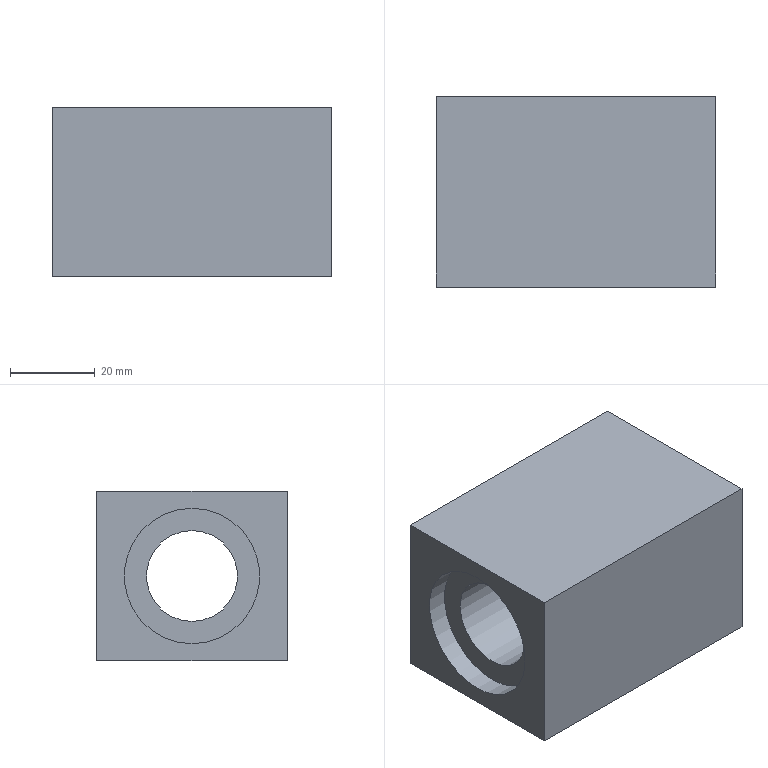Part | STEP file | Tube feed_id826_x_t | 1 solid | 23 faces | box 66 x 45 x 40 mm | volume 90173 mm3 | plane 8 | cone 8 | cylinder 7 | commonest cylinder face diameters 3.3 x4 32 x2 21.5 x1
STEP:
#1=CARTESIAN_POINT('',(0.,0.,0.));
#2=DIRECTION('',(0.,0.,1.));
#3=DIRECTION('',(1.,0.,0.));
#4=AXIS2_PLACEMENT_3D('',#1,#2,#3);
#5=CARTESIAN_POINT('',(-554.,10.056,44.373));
#6=VERTEX_POINT('',#5);
#7=CARTESIAN_POINT('',(-554.,10.056,28.373));
#8=DIRECTION('',(-1.,0.,0.));
#9=DIRECTION('',(0.,0.,1.));
#10=AXIS2_PLACEMENT_3D('',#7,#8,#9);
#11=CIRCLE('',#10,16.);
#12=CARTESIAN_POINT('',(-554.,-12.444,8.1));
#13=DIRECTION('',(1.,0.,0.));
#14=DIRECTION('',(0.,0.,-1.));
#15=AXIS2_PLACEMENT_3D('',#12,#13,#14);
#16=PLANE('',#15);
#17=CARTESIAN_POINT('',(-36.273,22.5));
#18=CARTESIAN_POINT('',(-36.273,50.213));
#19=CARTESIAN_POINT('',(-12.273,36.356));
#20=CARTESIAN_POINT('',(11.727,22.5));
#21=CARTESIAN_POINT('',(-12.273,8.644));
#22=CARTESIAN_POINT('',(-36.273,-5.213));
#23=CARTESIAN_POINT('',(-36.273,22.5));
#24=(BOUNDED_CURVE()B_SPLINE_CURVE(2,(#17,#18,#19,#20,#21,#22,#23),.UNSPECIFIED.,.T.,.F.)B_SPLINE_CURVE_WITH_KNOTS((1,2,2,2,2,1),(-2.094,0.,2.094,4.189,6.283,8.378),.UNSPECIFIED.)CURVE()GEOMETRIC_REPRESENTATION_ITEM()RATIONAL_B_SPLINE_CURVE((1.,0.5,1.,0.5,1.,0.5,1.))REPRESENTATION_ITEM(''));
#25=(GEOMETRIC_REPRESENTATION_CONTEXT(2)PARAMETRIC_REPRESENTATION_CONTEXT()REPRESENTATION_CONTEXT('',''));
#26=DEFINITIONAL_REPRESENTATION('',(#24),#25);
#27=PCURVE('',#16,#26);
#28=CARTESIAN_POINT('',(-554.,10.056,28.373));
#29=DIRECTION('',(-1.,0.,0.));
#30=DIRECTION('',(0.,0.,1.));
#31=AXIS2_PLACEMENT_3D('',#28,#29,#30);
#32=CYLINDRICAL_SURFACE('',#31,16.);
#33=CARTESIAN_POINT('',(0.,0.));
#34=DIRECTION('',(1.,0.));
#35=VECTOR('',#34,1.);
#36=LINE('',#33,#35);
#37=(GEOMETRIC_REPRESENTATION_CONTEXT(2)PARAMETRIC_REPRESENTATION_CONTEXT()REPRESENTATION_CONTEXT('',''));
#38=DEFINITIONAL_REPRESENTATION('',(#36),#37);
#39=PCURVE('',#32,#38);
#40=SURFACE_CURVE('',#11,(#27,#39),.PCURVE_S1.);
#41=EDGE_CURVE('',#6,#6,#40,.T.);
#42=ORIENTED_EDGE('',*,*,#41,.T.);
#43=EDGE_LOOP('',(#42));
#44=FACE_BOUND('',#43,.T.);
#45=CARTESIAN_POINT('',(-554.,-12.444,48.1));
#46=VERTEX_POINT('',#45);
#47=CARTESIAN_POINT('',(-554.,32.556,48.1));
#48=VERTEX_POINT('',#47);
#49=CARTESIAN_POINT('',(-554.,-12.444,48.1));
#50=DIRECTION('',(0.,1.,0.));
#51=VECTOR('',#50,1.);
#52=LINE('',#49,#51);
#53=CARTESIAN_POINT('',(-40.,0.));
#54=DIRECTION('',(0.,1.));
#55=VECTOR('',#54,1.);
#56=LINE('',#53,#55);
#57=(GEOMETRIC_REPRESENTATION_CONTEXT(2)PARAMETRIC_REPRESENTATION_CONTEXT()REPRESENTATION_CONTEXT('',''));
#58=DEFINITIONAL_REPRESENTATION('',(#56),#57);
#59=PCURVE('',#16,#58);
#60=CARTESIAN_POINT('',(-150.,0.,48.1));
#61=DIRECTION('',(0.,0.,1.));
#62=DIRECTION('',(1.,0.,0.));
#63=AXIS2_PLACEMENT_3D('',#60,#61,#62);
#64=PLANE('',#63);
#65=CARTESIAN_POINT('',(-404.,-12.444));
#66=DIRECTION('',(0.,1.));
#67=VECTOR('',#66,1.);
#68=LINE('',#65,#67);
#69=(GEOMETRIC_REPRESENTATION_CONTEXT(2)PARAMETRIC_REPRESENTATION_CONTEXT()REPRESENTATION_CONTEXT('',''));
#70=DEFINITIONAL_REPRESENTATION('',(#68),#69);
#71=PCURVE('',#64,#70);
#72=SURFACE_CURVE('',#52,(#59,#71),.PCURVE_S1.);
#73=EDGE_CURVE('',#46,#48,#72,.T.);
#74=ORIENTED_EDGE('',*,*,#73,.F.);
#75=CARTESIAN_POINT('',(-554.,-12.444,8.1));
#76=VERTEX_POINT('',#75);
#77=CARTESIAN_POINT('',(-554.,-12.444,8.1));
#78=DIRECTION('',(0.,0.,1.));
#79=VECTOR('',#78,1.);
#80=LINE('',#77,#79);
#81=CARTESIAN_POINT('',(0.,0.));
#82=DIRECTION('',(-1.,0.));
#83=VECTOR('',#82,1.);
#84=LINE('',#81,#83);
#85=(GEOMETRIC_REPRESENTATION_CONTEXT(2)PARAMETRIC_REPRESENTATION_CONTEXT()REPRESENTATION_CONTEXT('',''));
#86=DEFINITIONAL_REPRESENTATION('',(#84),#85);
#87=PCURVE('',#16,#86);
#88=CARTESIAN_POINT('',(-620.,-12.444,8.1));
#89=DIRECTION('',(0.,-1.,0.));
#90=DIRECTION('',(0.,0.,-1.));
#91=AXIS2_PLACEMENT_3D('',#88,#89,#90);
#92=PLANE('',#91);
#93=CARTESIAN_POINT('',(0.,66.));
#94=DIRECTION('',(-1.,0.));
#95=VECTOR('',#94,1.);
#96=LINE('',#93,#95);
#97=(GEOMETRIC_REPRESENTATION_CONTEXT(2)PARAMETRIC_REPRESENTATION_CONTEXT()REPRESENTATION_CONTEXT('',''));
#98=DEFINITIONAL_REPRESENTATION('',(#96),#97);
#99=PCURVE('',#92,#98);
#100=SURFACE_CURVE('',#80,(#87,#99),.PCURVE_S1.);
#101=EDGE_CURVE('',#76,#46,#100,.T.);
#102=ORIENTED_EDGE('',*,*,#101,.F.);
#103=CARTESIAN_POINT('',(-554.,32.556,8.1));
#104=VERTEX_POINT('',#103);
#105=CARTESIAN_POINT('',(-554.,-12.444,8.1));
#106=DIRECTION('',(0.,1.,0.));
#107=VECTOR('',#106,1.);
#108=LINE('',#105,#107);
#109=CARTESIAN_POINT('',(0.,0.));
#110=DIRECTION('',(0.,1.));
#111=VECTOR('',#110,1.);
#112=LINE('',#109,#111);
#113=(GEOMETRIC_REPRESENTATION_CONTEXT(2)PARAMETRIC_REPRESENTATION_CONTEXT()REPRESENTATION_CONTEXT('',''));
#114=DEFINITIONAL_REPRESENTATION('',(#112),#113);
#115=PCURVE('',#16,#114);
#116=CARTESIAN_POINT('',(-150.,0.,8.1));
#117=DIRECTION('',(0.,0.,1.));
#118=DIRECTION('',(1.,0.,0.));
#119=AXIS2_PLACEMENT_3D('',#116,#117,#118);
#120=PLANE('',#119);
#121=CARTESIAN_POINT('',(-404.,-12.444));
#122=DIRECTION('',(0.,1.));
#123=VECTOR('',#122,1.);
#124=LINE('',#121,#123);
#125=(GEOMETRIC_REPRESENTATION_CONTEXT(2)PARAMETRIC_REPRESENTATION_CONTEXT()REPRESENTATION_CONTEXT('',''));
#126=DEFINITIONAL_REPRESENTATION('',(#124),#125);
#127=PCURVE('',#120,#126);
#128=SURFACE_CURVE('',#108,(#115,#127),.PCURVE_S1.);
#129=EDGE_CURVE('',#76,#104,#128,.T.);
#130=ORIENTED_EDGE('',*,*,#129,.T.);
#131=CARTESIAN_POINT('',(-554.,32.556,8.1));
#132=DIRECTION('',(0.,0.,1.));
#133=VECTOR('',#132,1.);
#134=LINE('',#131,#133);
#135=CARTESIAN_POINT('',(0.,45.));
#136=DIRECTION('',(-1.,0.));
#137=VECTOR('',#136,1.);
#138=LINE('',#135,#137);
#139=(GEOMETRIC_REPRESENTATION_CONTEXT(2)PARAMETRIC_REPRESENTATION_CONTEXT()REPRESENTATION_CONTEXT('',''));
#140=DEFINITIONAL_REPRESENTATION('',(#138),#139);
#141=PCURVE('',#16,#140);
#142=CARTESIAN_POINT('',(-554.,32.556,8.1));
#143=DIRECTION('',(0.,1.,0.));
#144=DIRECTION('',(0.,0.,1.));
#145=AXIS2_PLACEMENT_3D('',#142,#143,#144);
#146=PLANE('',#145);
#147=CARTESIAN_POINT('',(0.,0.));
#148=DIRECTION('',(1.,0.));
#149=VECTOR('',#148,1.);
#150=LINE('',#147,#149);
#151=(GEOMETRIC_REPRESENTATION_CONTEXT(2)PARAMETRIC_REPRESENTATION_CONTEXT()REPRESENTATION_CONTEXT('',''));
#152=DEFINITIONAL_REPRESENTATION('',(#150),#151);
#153=PCURVE('',#146,#152);
#154=SURFACE_CURVE('',#134,(#141,#153),.PCURVE_S1.);
#155=EDGE_CURVE('',#104,#48,#154,.T.);
#156=ORIENTED_EDGE('',*,*,#155,.T.);
#157=EDGE_LOOP('',(#74,#102,#130,#156));
#158=FACE_BOUND('',#157,.T.);
#159=ADVANCED_FACE('',(#44,#158),#16,.T.);
#160=CARTESIAN_POINT('',(-620.,32.556,48.1));
#161=VERTEX_POINT('',#160);
#162=CARTESIAN_POINT('',(-554.,32.556,48.1));
#163=DIRECTION('',(-1.,0.,0.));
#164=VECTOR('',#163,1.);
#165=LINE('',#162,#164);
#166=CARTESIAN_POINT('',(40.,0.));
#167=DIRECTION('',(0.,-1.));
#168=VECTOR('',#167,1.);
#169=LINE('',#166,#168);
#170=(GEOMETRIC_REPRESENTATION_CONTEXT(2)PARAMETRIC_REPRESENTATION_CONTEXT()REPRESENTATION_CONTEXT('',''));
#171=DEFINITIONAL_REPRESENTATION('',(#169),#170);
#172=PCURVE('',#146,#171);
#173=CARTESIAN_POINT('',(-404.,32.556));
#174=DIRECTION('',(-1.,0.));
#175=VECTOR('',#174,1.);
#176=LINE('',#173,#175);
#177=(GEOMETRIC_REPRESENTATION_CONTEXT(2)PARAMETRIC_REPRESENTATION_CONTEXT()REPRESENTATION_CONTEXT('',''));
#178=DEFINITIONAL_REPRESENTATION('',(#176),#177);
#179=PCURVE('',#64,#178);
#180=SURFACE_CURVE('',#165,(#172,#179),.PCURVE_S1.);
#181=EDGE_CURVE('',#48,#161,#180,.T.);
#182=ORIENTED_EDGE('',*,*,#181,.F.);
#183=ORIENTED_EDGE('',*,*,#155,.F.);
#184=CARTESIAN_POINT('',(-620.,32.556,8.1));
#185=VERTEX_POINT('',#184);
#186=CARTESIAN_POINT('',(-554.,32.556,8.1));
#187=DIRECTION('',(-1.,0.,0.));
#188=VECTOR('',#187,1.);
#189=LINE('',#186,#188);
#190=CARTESIAN_POINT('',(0.,0.));
#191=DIRECTION('',(0.,-1.));
#192=VECTOR('',#191,1.);
#193=LINE('',#190,#192);
#194=(GEOMETRIC_REPRESENTATION_CONTEXT(2)PARAMETRIC_REPRESENTATION_CONTEXT()REPRESENTATION_CONTEXT('',''));
#195=DEFINITIONAL_REPRESENTATION('',(#193),#194);
#196=PCURVE('',#146,#195);
#197=CARTESIAN_POINT('',(-404.,32.556));
#198=DIRECTION('',(-1.,0.));
#199=VECTOR('',#198,1.);
#200=LINE('',#197,#199);
#201=(GEOMETRIC_REPRESENTATION_CONTEXT(2)PARAMETRIC_REPRESENTATION_CONTEXT()REPRESENTATION_CONTEXT('',''));
#202=DEFINITIONAL_REPRESENTATION('',(#200),#201);
#203=PCURVE('',#120,#202);
#204=SURFACE_CURVE('',#189,(#196,#203),.PCURVE_S1.);
#205=EDGE_CURVE('',#104,#185,#204,.T.);
#206=ORIENTED_EDGE('',*,*,#205,.T.);
#207=CARTESIAN_POINT('',(-620.,32.556,8.1));
#208=DIRECTION('',(0.,0.,1.));
#209=VECTOR('',#208,1.);
#210=LINE('',#207,#209);
#211=CARTESIAN_POINT('',(0.,-66.));
#212=DIRECTION('',(1.,0.));
#213=VECTOR('',#212,1.);
#214=LINE('',#211,#213);
#215=(GEOMETRIC_REPRESENTATION_CONTEXT(2)PARAMETRIC_REPRESENTATION_CONTEXT()REPRESENTATION_CONTEXT('',''));
#216=DEFINITIONAL_REPRESENTATION('',(#214),#215);
#217=PCURVE('',#146,#216);
#218=CARTESIAN_POINT('',(-620.,32.556,8.1));
#219=DIRECTION('',(-1.,0.,0.));
#220=DIRECTION('',(0.,0.,1.));
#221=AXIS2_PLACEMENT_3D('',#218,#219,#220);
#222=PLANE('',#221);
#223=CARTESIAN_POINT('',(0.,0.));
#224=DIRECTION('',(1.,0.));
#225=VECTOR('',#224,1.);
#226=LINE('',#223,#225);
#227=(GEOMETRIC_REPRESENTATION_CONTEXT(2)PARAMETRIC_REPRESENTATION_CONTEXT()REPRESENTATION_CONTEXT('',''));
#228=DEFINITIONAL_REPRESENTATION('',(#226),#227);
#229=PCURVE('',#222,#228);
#230=SURFACE_CURVE('',#210,(#217,#229),.PCURVE_S1.);
#231=EDGE_CURVE('',#185,#161,#230,.T.);
#232=ORIENTED_EDGE('',*,*,#231,.T.);
#233=EDGE_LOOP('',(#182,#183,#206,#232));
#234=FACE_BOUND('',#233,.T.);
#235=ADVANCED_FACE('',(#234),#146,.T.);
#236=CARTESIAN_POINT('',(-620.,10.056,12.1));
#237=VERTEX_POINT('',#236);
#238=CARTESIAN_POINT('',(-620.,10.056,28.1));
#239=DIRECTION('',(1.,0.,0.));
#240=DIRECTION('',(0.,0.,-1.));
#241=AXIS2_PLACEMENT_3D('',#238,#239,#240);
#242=CIRCLE('',#241,16.);
#243=CARTESIAN_POINT('',(4.,-22.5));
#244=CARTESIAN_POINT('',(4.,5.213));
#245=CARTESIAN_POINT('',(28.,-8.644));
#246=CARTESIAN_POINT('',(52.,-22.5));
#247=CARTESIAN_POINT('',(28.,-36.356));
#248=CARTESIAN_POINT('',(4.,-50.213));
#249=CARTESIAN_POINT('',(4.,-22.5));
#250=(BOUNDED_CURVE()B_SPLINE_CURVE(2,(#243,#244,#245,#246,#247,#248,#249),.UNSPECIFIED.,.T.,.F.)B_SPLINE_CURVE_WITH_KNOTS((1,2,2,2,2,1),(-2.094,0.,2.094,4.189,6.283,8.378),.UNSPECIFIED.)CURVE()GEOMETRIC_REPRESENTATION_ITEM()RATIONAL_B_SPLINE_CURVE((1.,0.5,1.,0.5,1.,0.5,1.))REPRESENTATION_ITEM(''));
#251=(GEOMETRIC_REPRESENTATION_CONTEXT(2)PARAMETRIC_REPRESENTATION_CONTEXT()REPRESENTATION_CONTEXT('',''));
#252=DEFINITIONAL_REPRESENTATION('',(#250),#251);
#253=PCURVE('',#222,#252);
#254=CARTESIAN_POINT('',(-620.,10.056,28.1));
#255=DIRECTION('',(1.,0.,0.));
#256=DIRECTION('',(0.,0.,-1.));
#257=AXIS2_PLACEMENT_3D('',#254,#255,#256);
#258=CYLINDRICAL_SURFACE('',#257,16.);
#259=CARTESIAN_POINT('',(0.,0.));
#260=DIRECTION('',(1.,0.));
#261=VECTOR('',#260,1.);
#262=LINE('',#259,#261);
#263=(GEOMETRIC_REPRESENTATION_CONTEXT(2)PARAMETRIC_REPRESENTATION_CONTEXT()REPRESENTATION_CONTEXT('',''));
#264=DEFINITIONAL_REPRESENTATION('',(#262),#263);
#265=PCURVE('',#258,#264);
#266=SURFACE_CURVE('',#242,(#253,#265),.PCURVE_S1.);
#267=EDGE_CURVE('',#237,#237,#266,.T.);
#268=ORIENTED_EDGE('',*,*,#267,.T.);
#269=EDGE_LOOP('',(#268));
#270=FACE_BOUND('',#269,.T.);
#271=CARTESIAN_POINT('',(-620.,-12.444,48.1));
#272=VERTEX_POINT('',#271);
#273=CARTESIAN_POINT('',(-620.,32.556,48.1));
#274=DIRECTION('',(0.,-1.,0.));
#275=VECTOR('',#274,1.);
#276=LINE('',#273,#275);
#277=CARTESIAN_POINT('',(40.,0.));
#278=DIRECTION('',(0.,-1.));
#279=VECTOR('',#278,1.);
#280=LINE('',#277,#279);
#281=(GEOMETRIC_REPRESENTATION_CONTEXT(2)PARAMETRIC_REPRESENTATION_CONTEXT()REPRESENTATION_CONTEXT('',''));
#282=DEFINITIONAL_REPRESENTATION('',(#280),#281);
#283=PCURVE('',#222,#282);
#284=CARTESIAN_POINT('',(-470.,32.556));
#285=DIRECTION('',(0.,-1.));
#286=VECTOR('',#285,1.);
#287=LINE('',#284,#286);
#288=(GEOMETRIC_REPRESENTATION_CONTEXT(2)PARAMETRIC_REPRESENTATION_CONTEXT()REPRESENTATION_CONTEXT('',''));
#289=DEFINITIONAL_REPRESENTATION('',(#287),#288);
#290=PCURVE('',#64,#289);
#291=SURFACE_CURVE('',#276,(#283,#290),.PCURVE_S1.);
#292=EDGE_CURVE('',#161,#272,#291,.T.);
#293=ORIENTED_EDGE('',*,*,#292,.F.);
#294=ORIENTED_EDGE('',*,*,#231,.F.);
#295=CARTESIAN_POINT('',(-620.,-12.444,8.1));
#296=VERTEX_POINT('',#295);
#297=CARTESIAN_POINT('',(-620.,32.556,8.1));
#298=DIRECTION('',(0.,-1.,0.));
#299=VECTOR('',#298,1.);
#300=LINE('',#297,#299);
#301=CARTESIAN_POINT('',(0.,0.));
#302=DIRECTION('',(0.,-1.));
#303=VECTOR('',#302,1.);
#304=LINE('',#301,#303);
#305=(GEOMETRIC_REPRESENTATION_CONTEXT(2)PARAMETRIC_REPRESENTATION_CONTEXT()REPRESENTATION_CONTEXT('',''));
#306=DEFINITIONAL_REPRESENTATION('',(#304),#305);
#307=PCURVE('',#222,#306);
#308=CARTESIAN_POINT('',(-470.,32.556));
#309=DIRECTION('',(0.,-1.));
#310=VECTOR('',#309,1.);
#311=LINE('',#308,#310);
#312=(GEOMETRIC_REPRESENTATION_CONTEXT(2)PARAMETRIC_REPRESENTATION_CONTEXT()REPRESENTATION_CONTEXT('',''));
#313=DEFINITIONAL_REPRESENTATION('',(#311),#312);
#314=PCURVE('',#120,#313);
#315=SURFACE_CURVE('',#300,(#307,#314),.PCURVE_S1.);
#316=EDGE_CURVE('',#185,#296,#315,.T.);
#317=ORIENTED_EDGE('',*,*,#316,.T.);
#318=CARTESIAN_POINT('',(-620.,-12.444,8.1));
#319=DIRECTION('',(0.,0.,1.));
#320=VECTOR('',#319,1.);
#321=LINE('',#318,#320);
#322=CARTESIAN_POINT('',(0.,-45.));
#323=DIRECTION('',(1.,0.));
#324=VECTOR('',#323,1.);
#325=LINE('',#322,#324);
#326=(GEOMETRIC_REPRESENTATION_CONTEXT(2)PARAMETRIC_REPRESENTATION_CONTEXT()REPRESENTATION_CONTEXT('',''));
#327=DEFINITIONAL_REPRESENTATION('',(#325),#326);
#328=PCURVE('',#222,#327);
#329=CARTESIAN_POINT('',(0.,0.));
#330=DIRECTION('',(-1.,0.));
#331=VECTOR('',#330,1.);
#332=LINE('',#329,#331);
#333=(GEOMETRIC_REPRESENTATION_CONTEXT(2)PARAMETRIC_REPRESENTATION_CONTEXT()REPRESENTATION_CONTEXT('',''));
#334=DEFINITIONAL_REPRESENTATION('',(#332),#333);
#335=PCURVE('',#92,#334);
#336=SURFACE_CURVE('',#321,(#328,#335),.PCURVE_S1.);
#337=EDGE_CURVE('',#296,#272,#336,.T.);
#338=ORIENTED_EDGE('',*,*,#337,.T.);
#339=EDGE_LOOP('',(#293,#294,#317,#338));
#340=FACE_BOUND('',#339,.T.);
#341=ADVANCED_FACE('',(#270,#340),#222,.T.);
#342=CARTESIAN_POINT('',(-620.,-12.444,48.1));
#343=DIRECTION('',(1.,0.,0.));
#344=VECTOR('',#343,1.);
#345=LINE('',#342,#344);
#346=CARTESIAN_POINT('',(-40.,0.));
#347=DIRECTION('',(0.,1.));
#348=VECTOR('',#347,1.);
#349=LINE('',#346,#348);
#350=(GEOMETRIC_REPRESENTATION_CONTEXT(2)PARAMETRIC_REPRESENTATION_CONTEXT()REPRESENTATION_CONTEXT('',''));
#351=DEFINITIONAL_REPRESENTATION('',(#349),#350);
#352=PCURVE('',#92,#351);
#353=CARTESIAN_POINT('',(-470.,-12.444));
#354=DIRECTION('',(1.,0.));
#355=VECTOR('',#354,1.);
#356=LINE('',#353,#355);
#357=(GEOMETRIC_REPRESENTATION_CONTEXT(2)PARAMETRIC_REPRESENTATION_CONTEXT()REPRESENTATION_CONTEXT('',''));
#358=DEFINITIONAL_REPRESENTATION('',(#356),#357);
#359=PCURVE('',#64,#358);
#360=SURFACE_CURVE('',#345,(#352,#359),.PCURVE_S1.);
#361=EDGE_CURVE('',#272,#46,#360,.T.);
#362=ORIENTED_EDGE('',*,*,#361,.F.);
#363=ORIENTED_EDGE('',*,*,#337,.F.);
#364=CARTESIAN_POINT('',(-620.,-12.444,8.1));
#365=DIRECTION('',(1.,0.,0.));
#366=VECTOR('',#365,1.);
#367=LINE('',#364,#366);
#368=CARTESIAN_POINT('',(0.,0.));
#369=DIRECTION('',(0.,1.));
#370=VECTOR('',#369,1.);
#371=LINE('',#368,#370);
#372=(GEOMETRIC_REPRESENTATION_CONTEXT(2)PARAMETRIC_REPRESENTATION_CONTEXT()REPRESENTATION_CONTEXT('',''));
#373=DEFINITIONAL_REPRESENTATION('',(#371),#372);
#374=PCURVE('',#92,#373);
#375=CARTESIAN_POINT('',(-470.,-12.444));
#376=DIRECTION('',(1.,0.));
#377=VECTOR('',#376,1.);
#378=LINE('',#375,#377);
#379=(GEOMETRIC_REPRESENTATION_CONTEXT(2)PARAMETRIC_REPRESENTATION_CONTEXT()REPRESENTATION_CONTEXT('',''));
#380=DEFINITIONAL_REPRESENTATION('',(#378),#379);
#381=PCURVE('',#120,#380);
#382=SURFACE_CURVE('',#367,(#374,#381),.PCURVE_S1.);
#383=EDGE_CURVE('',#296,#76,#382,.T.);
#384=ORIENTED_EDGE('',*,*,#383,.T.);
#385=ORIENTED_EDGE('',*,*,#101,.T.);
#386=EDGE_LOOP('',(#362,#363,#384,#385));
#387=FACE_BOUND('',#386,.T.);
#388=ADVANCED_FACE('',(#387),#92,.T.);
#389=CARTESIAN_POINT('',(-610.,22.556,8.1));
#390=VERTEX_POINT('',#389);
#391=CARTESIAN_POINT('',(-612.,22.556,8.1));
#392=DIRECTION('',(0.,0.,1.));
#393=DIRECTION('',(1.,0.,0.));
#394=AXIS2_PLACEMENT_3D('',#391,#392,#393);
#395=CIRCLE('',#394,2.);
#396=CARTESIAN_POINT('',(-462.,22.556));
#397=DIRECTION('',(1.,0.));
#398=AXIS2_PLACEMENT_2D('',#396,#397);
#399=CIRCLE('',#398,2.);
#400=(GEOMETRIC_REPRESENTATION_CONTEXT(2)PARAMETRIC_REPRESENTATION_CONTEXT()REPRESENTATION_CONTEXT('',''));
#401=DEFINITIONAL_REPRESENTATION('',(#399),#400);
#402=PCURVE('',#120,#401);
#403=CARTESIAN_POINT('',(-612.,22.556,8.1));
#404=DIRECTION('',(0.,0.,-1.));
#405=DIRECTION('',(-1.,0.,0.));
#406=AXIS2_PLACEMENT_3D('',#403,#404,#405);
#407=CONICAL_SURFACE('',#406,2.,0.7854);
#408=CARTESIAN_POINT('',(9.425,0.));
#409=DIRECTION('',(-1.,0.));
#410=VECTOR('',#409,1.);
#411=LINE('',#408,#410);
#412=(GEOMETRIC_REPRESENTATION_CONTEXT(2)PARAMETRIC_REPRESENTATION_CONTEXT()REPRESENTATION_CONTEXT('',''));
#413=DEFINITIONAL_REPRESENTATION('',(#411),#412);
#414=PCURVE('',#407,#413);
#415=SURFACE_CURVE('',#395,(#402,#414),.PCURVE_S1.);
#416=EDGE_CURVE('',#390,#390,#415,.T.);
#417=ORIENTED_EDGE('',*,*,#416,.T.);
#418=EDGE_LOOP('',(#417));
#419=FACE_BOUND('',#418,.T.);
#420=CARTESIAN_POINT('',(-560.,22.556,8.1));
#421=VERTEX_POINT('',#420);
#422=CARTESIAN_POINT('',(-562.,22.556,8.1));
#423=DIRECTION('',(0.,0.,1.));
#424=DIRECTION('',(1.,0.,0.));
#425=AXIS2_PLACEMENT_3D('',#422,#423,#424);
#426=CIRCLE('',#425,2.);
#427=CARTESIAN_POINT('',(-412.,22.556));
#428=DIRECTION('',(1.,0.));
#429=AXIS2_PLACEMENT_2D('',#427,#428);
#430=CIRCLE('',#429,2.);
#431=(GEOMETRIC_REPRESENTATION_CONTEXT(2)PARAMETRIC_REPRESENTATION_CONTEXT()REPRESENTATION_CONTEXT('',''));
#432=DEFINITIONAL_REPRESENTATION('',(#430),#431);
#433=PCURVE('',#120,#432);
#434=CARTESIAN_POINT('',(-562.,22.556,8.1));
#435=DIRECTION('',(0.,0.,-1.));
#436=DIRECTION('',(-1.,0.,0.));
#437=AXIS2_PLACEMENT_3D('',#434,#435,#436);
#438=CONICAL_SURFACE('',#437,2.,0.7854);
#439=CARTESIAN_POINT('',(9.425,0.));
#440=DIRECTION('',(-1.,0.));
#441=VECTOR('',#440,1.);
#442=LINE('',#439,#441);
#443=(GEOMETRIC_REPRESENTATION_CONTEXT(2)PARAMETRIC_REPRESENTATION_CONTEXT()REPRESENTATION_CONTEXT('',''));
#444=DEFINITIONAL_REPRESENTATION('',(#442),#443);
#445=PCURVE('',#438,#444);
#446=SURFACE_CURVE('',#426,(#433,#445),.PCURVE_S1.);
#447=EDGE_CURVE('',#421,#421,#446,.T.);
#448=ORIENTED_EDGE('',*,*,#447,.T.);
#449=EDGE_LOOP('',(#448));
#450=FACE_BOUND('',#449,.T.);
#451=CARTESIAN_POINT('',(-560.,-2.444,8.1));
#452=VERTEX_POINT('',#451);
#453=CARTESIAN_POINT('',(-562.,-2.444,8.1));
#454=DIRECTION('',(0.,0.,1.));
#455=DIRECTION('',(1.,0.,0.));
#456=AXIS2_PLACEMENT_3D('',#453,#454,#455);
#457=CIRCLE('',#456,2.);
#458=CARTESIAN_POINT('',(-412.,-2.444));
#459=DIRECTION('',(1.,0.));
#460=AXIS2_PLACEMENT_2D('',#458,#459);
#461=CIRCLE('',#460,2.);
#462=(GEOMETRIC_REPRESENTATION_CONTEXT(2)PARAMETRIC_REPRESENTATION_CONTEXT()REPRESENTATION_CONTEXT('',''));
#463=DEFINITIONAL_REPRESENTATION('',(#461),#462);
#464=PCURVE('',#120,#463);
#465=CARTESIAN_POINT('',(-562.,-2.444,8.1));
#466=DIRECTION('',(0.,0.,-1.));
#467=DIRECTION('',(-1.,0.,0.));
#468=AXIS2_PLACEMENT_3D('',#465,#466,#467);
#469=CONICAL_SURFACE('',#468,2.,0.7854);
#470=CARTESIAN_POINT('',(9.425,0.));
#471=DIRECTION('',(-1.,0.));
#472=VECTOR('',#471,1.);
#473=LINE('',#470,#472);
#474=(GEOMETRIC_REPRESENTATION_CONTEXT(2)PARAMETRIC_REPRESENTATION_CONTEXT()REPRESENTATION_CONTEXT('',''));
#475=DEFINITIONAL_REPRESENTATION('',(#473),#474);
#476=PCURVE('',#469,#475);
#477=SURFACE_CURVE('',#457,(#464,#476),.PCURVE_S1.);
#478=EDGE_CURVE('',#452,#452,#477,.T.);
#479=ORIENTED_EDGE('',*,*,#478,.T.);
#480=EDGE_LOOP('',(#479));
#481=FACE_BOUND('',#480,.T.);
#482=CARTESIAN_POINT('',(-610.,-2.444,8.1));
#483=VERTEX_POINT('',#482);
#484=CARTESIAN_POINT('',(-612.,-2.444,8.1));
#485=DIRECTION('',(0.,0.,1.));
#486=DIRECTION('',(1.,0.,0.));
#487=AXIS2_PLACEMENT_3D('',#484,#485,#486);
#488=CIRCLE('',#487,2.);
#489=CARTESIAN_POINT('',(-462.,-2.444));
#490=DIRECTION('',(1.,0.));
#491=AXIS2_PLACEMENT_2D('',#489,#490);
#492=CIRCLE('',#491,2.);
#493=(GEOMETRIC_REPRESENTATION_CONTEXT(2)PARAMETRIC_REPRESENTATION_CONTEXT()REPRESENTATION_CONTEXT('',''));
#494=DEFINITIONAL_REPRESENTATION('',(#492),#493);
#495=PCURVE('',#120,#494);
#496=CARTESIAN_POINT('',(-612.,-2.444,8.1));
#497=DIRECTION('',(0.,0.,-1.));
#498=DIRECTION('',(-1.,0.,0.));
#499=AXIS2_PLACEMENT_3D('',#496,#497,#498);
#500=CONICAL_SURFACE('',#499,2.,0.7854);
#501=CARTESIAN_POINT('',(9.425,0.));
#502=DIRECTION('',(-1.,0.));
#503=VECTOR('',#502,1.);
#504=LINE('',#501,#503);
#505=(GEOMETRIC_REPRESENTATION_CONTEXT(2)PARAMETRIC_REPRESENTATION_CONTEXT()REPRESENTATION_CONTEXT('',''));
#506=DEFINITIONAL_REPRESENTATION('',(#504),#505);
#507=PCURVE('',#500,#506);
#508=SURFACE_CURVE('',#488,(#495,#507),.PCURVE_S1.);
#509=EDGE_CURVE('',#483,#483,#508,.T.);
#510=ORIENTED_EDGE('',*,*,#509,.T.);
#511=EDGE_LOOP('',(#510));
#512=FACE_BOUND('',#511,.T.);
#513=ORIENTED_EDGE('',*,*,#129,.F.);
#514=ORIENTED_EDGE('',*,*,#383,.F.);
#515=ORIENTED_EDGE('',*,*,#316,.F.);
#516=ORIENTED_EDGE('',*,*,#205,.F.);
#517=EDGE_LOOP('',(#513,#514,#515,#516));
#518=FACE_BOUND('',#517,.T.);
#519=ADVANCED_FACE('',(#419,#450,#481,#512,#518),#120,.F.);
#520=ORIENTED_EDGE('',*,*,#73,.T.);
#521=ORIENTED_EDGE('',*,*,#181,.T.);
#522=ORIENTED_EDGE('',*,*,#292,.T.);
#523=ORIENTED_EDGE('',*,*,#361,.T.);
#524=EDGE_LOOP('',(#520,#521,#522,#523));
#525=FACE_BOUND('',#524,.T.);
#526=ADVANCED_FACE('',(#525),#64,.T.);
#527=CARTESIAN_POINT('',(-559.,10.056,38.85));
#528=VERTEX_POINT('',#527);
#529=CARTESIAN_POINT('',(-559.,10.056,17.35));
#530=VERTEX_POINT('',#529);
#531=CARTESIAN_POINT('',(-559.,10.056,28.1));
#532=DIRECTION('',(-1.,0.,0.));
#533=DIRECTION('',(0.,0.,1.));
#534=AXIS2_PLACEMENT_3D('',#531,#532,#533);
#535=CIRCLE('',#534,10.75);
#536=CARTESIAN_POINT('',(-559.,10.056,28.373));
#537=DIRECTION('',(-1.,0.,0.));
#538=DIRECTION('',(0.,0.,1.));
#539=AXIS2_PLACEMENT_3D('',#536,#537,#538);
#540=PLANE('',#539);
#541=CARTESIAN_POINT('',(-0.2729,0.));
#542=DIRECTION('',(1.,0.));
#543=AXIS2_PLACEMENT_2D('',#541,#542);
#544=CIRCLE('',#543,10.75);
#545=(GEOMETRIC_REPRESENTATION_CONTEXT(2)PARAMETRIC_REPRESENTATION_CONTEXT()REPRESENTATION_CONTEXT('',''));
#546=DEFINITIONAL_REPRESENTATION('',(#544),#545);
#547=PCURVE('',#540,#546);
#548=CARTESIAN_POINT('',(-615.,10.056,28.1));
#549=DIRECTION('',(1.,0.,0.));
#550=DIRECTION('',(0.,0.,-1.));
#551=AXIS2_PLACEMENT_3D('',#548,#549,#550);
#552=CYLINDRICAL_SURFACE('',#551,10.75);
#553=CARTESIAN_POINT('',(3.142,56.));
#554=DIRECTION('',(-1.,0.));
#555=VECTOR('',#554,1.);
#556=LINE('',#553,#555);
#557=(GEOMETRIC_REPRESENTATION_CONTEXT(2)PARAMETRIC_REPRESENTATION_CONTEXT()REPRESENTATION_CONTEXT('',''));
#558=DEFINITIONAL_REPRESENTATION('',(#556),#557);
#559=PCURVE('',#552,#558);
#560=SURFACE_CURVE('',#535,(#547,#559),.PCURVE_S1.);
#561=EDGE_CURVE('',#528,#530,#560,.T.);
#562=ORIENTED_EDGE('',*,*,#561,.T.);
#563=CARTESIAN_POINT('',(-559.,10.056,28.1));
#564=DIRECTION('',(-1.,0.,0.));
#565=DIRECTION('',(0.,0.,1.));
#566=AXIS2_PLACEMENT_3D('',#563,#564,#565);
#567=CIRCLE('',#566,10.75);
#568=CARTESIAN_POINT('',(-0.2729,0.));
#569=DIRECTION('',(1.,0.));
#570=AXIS2_PLACEMENT_2D('',#568,#569);
#571=CIRCLE('',#570,10.75);
#572=(GEOMETRIC_REPRESENTATION_CONTEXT(2)PARAMETRIC_REPRESENTATION_CONTEXT()REPRESENTATION_CONTEXT('',''));
#573=DEFINITIONAL_REPRESENTATION('',(#571),#572);
#574=PCURVE('',#540,#573);
#575=CARTESIAN_POINT('',(9.425,56.));
#576=DIRECTION('',(-1.,0.));
#577=VECTOR('',#576,1.);
#578=LINE('',#575,#577);
#579=(GEOMETRIC_REPRESENTATION_CONTEXT(2)PARAMETRIC_REPRESENTATION_CONTEXT()REPRESENTATION_CONTEXT('',''));
#580=DEFINITIONAL_REPRESENTATION('',(#578),#579);
#581=PCURVE('',#552,#580);
#582=SURFACE_CURVE('',#567,(#574,#581),.PCURVE_S1.);
#583=EDGE_CURVE('',#530,#528,#582,.T.);
#584=ORIENTED_EDGE('',*,*,#583,.T.);
#585=EDGE_LOOP('',(#562,#584));
#586=FACE_BOUND('',#585,.T.);
#587=CARTESIAN_POINT('',(-559.,10.056,44.373));
#588=VERTEX_POINT('',#587);
#589=CARTESIAN_POINT('',(-559.,10.056,28.373));
#590=DIRECTION('',(-1.,0.,0.));
#591=DIRECTION('',(0.,0.,1.));
#592=AXIS2_PLACEMENT_3D('',#589,#590,#591);
#593=CIRCLE('',#592,16.);
#594=CARTESIAN_POINT('',(0.,0.));
#595=DIRECTION('',(1.,0.));
#596=AXIS2_PLACEMENT_2D('',#594,#595);
#597=CIRCLE('',#596,16.);
#598=(GEOMETRIC_REPRESENTATION_CONTEXT(2)PARAMETRIC_REPRESENTATION_CONTEXT()REPRESENTATION_CONTEXT('',''));
#599=DEFINITIONAL_REPRESENTATION('',(#597),#598);
#600=PCURVE('',#540,#599);
#601=CARTESIAN_POINT('',(0.,5.));
#602=DIRECTION('',(1.,0.));
#603=VECTOR('',#602,1.);
#604=LINE('',#601,#603);
#605=(GEOMETRIC_REPRESENTATION_CONTEXT(2)PARAMETRIC_REPRESENTATION_CONTEXT()REPRESENTATION_CONTEXT('',''));
#606=DEFINITIONAL_REPRESENTATION('',(#604),#605);
#607=PCURVE('',#32,#606);
#608=SURFACE_CURVE('',#593,(#600,#607),.PCURVE_S1.);
#609=EDGE_CURVE('',#588,#588,#608,.T.);
#610=ORIENTED_EDGE('',*,*,#609,.F.);
#611=EDGE_LOOP('',(#610));
#612=FACE_BOUND('',#611,.T.);
#613=ADVANCED_FACE('',(#586,#612),#540,.F.);
#614=ORIENTED_EDGE('',*,*,#609,.F.);
#615=CARTESIAN_POINT('',(-554.,10.056,44.373));
#616=CARTESIAN_POINT('',(-559.,10.056,44.373));
#617=B_SPLINE_CURVE_WITH_KNOTS('',1,(#615,#616),.UNSPECIFIED.,.F.,.F.,(2,2),(0.,5.),.PIECEWISE_BEZIER_KNOTS.);
#618=CARTESIAN_POINT('',(0.,0.));
#619=DIRECTION('',(0.,1.));
#620=VECTOR('',#619,1.);
#621=LINE('',#618,#620);
#622=(GEOMETRIC_REPRESENTATION_CONTEXT(2)PARAMETRIC_REPRESENTATION_CONTEXT()REPRESENTATION_CONTEXT('',''));
#623=DEFINITIONAL_REPRESENTATION('',(#621),#622);
#624=PCURVE('',#32,#623);
#625=CARTESIAN_POINT('',(6.283,0.));
#626=DIRECTION('',(0.,1.));
#627=VECTOR('',#626,1.);
#628=LINE('',#625,#627);
#629=(GEOMETRIC_REPRESENTATION_CONTEXT(2)PARAMETRIC_REPRESENTATION_CONTEXT()REPRESENTATION_CONTEXT('',''));
#630=DEFINITIONAL_REPRESENTATION('',(#628),#629);
#631=PCURVE('',#32,#630);
#632=SEAM_CURVE('',#617,(#624,#631),.PCURVE_S1.);
#633=EDGE_CURVE('',#6,#588,#632,.T.);
#634=ORIENTED_EDGE('',*,*,#633,.F.);
#635=ORIENTED_EDGE('',*,*,#41,.T.);
#636=ORIENTED_EDGE('',*,*,#633,.T.);
#637=EDGE_LOOP('',(#614,#634,#635,#636));
#638=FACE_BOUND('',#637,.F.);
#639=ADVANCED_FACE('',(#638),#32,.F.);
#640=CARTESIAN_POINT('',(-615.,10.056,17.35));
#641=VERTEX_POINT('',#640);
#642=CARTESIAN_POINT('',(-615.,10.056,28.1));
#643=DIRECTION('',(1.,0.,0.));
#644=DIRECTION('',(0.,0.,-1.));
#645=AXIS2_PLACEMENT_3D('',#642,#643,#644);
#646=CIRCLE('',#645,10.75);
#647=CARTESIAN_POINT('',(-615.,10.056,28.1));
#648=DIRECTION('',(1.,0.,0.));
#649=DIRECTION('',(0.,0.,-1.));
#650=AXIS2_PLACEMENT_3D('',#647,#648,#649);
#651=PLANE('',#650);
#652=CARTESIAN_POINT('',(0.,0.));
#653=DIRECTION('',(1.,0.));
#654=AXIS2_PLACEMENT_2D('',#652,#653);
#655=CIRCLE('',#654,10.75);
#656=(GEOMETRIC_REPRESENTATION_CONTEXT(2)PARAMETRIC_REPRESENTATION_CONTEXT()REPRESENTATION_CONTEXT('',''));
#657=DEFINITIONAL_REPRESENTATION('',(#655),#656);
#658=PCURVE('',#651,#657);
#659=CARTESIAN_POINT('',(0.,0.));
#660=DIRECTION('',(1.,0.));
#661=VECTOR('',#660,1.);
#662=LINE('',#659,#661);
#663=(GEOMETRIC_REPRESENTATION_CONTEXT(2)PARAMETRIC_REPRESENTATION_CONTEXT()REPRESENTATION_CONTEXT('',''));
#664=DEFINITIONAL_REPRESENTATION('',(#662),#663);
#665=PCURVE('',#552,#664);
#666=SURFACE_CURVE('',#646,(#658,#665),.PCURVE_S1.);
#667=EDGE_CURVE('',#641,#641,#666,.T.);
#668=ORIENTED_EDGE('',*,*,#667,.T.);
#669=EDGE_LOOP('',(#668));
#670=FACE_BOUND('',#669,.T.);
#671=CARTESIAN_POINT('',(-615.,10.056,12.1));
#672=VERTEX_POINT('',#671);
#673=CARTESIAN_POINT('',(-615.,10.056,28.1));
#674=DIRECTION('',(1.,0.,0.));
#675=DIRECTION('',(0.,0.,-1.));
#676=AXIS2_PLACEMENT_3D('',#673,#674,#675);
#677=CIRCLE('',#676,16.);
#678=CARTESIAN_POINT('',(0.,0.));
#679=DIRECTION('',(1.,0.));
#680=AXIS2_PLACEMENT_2D('',#678,#679);
#681=CIRCLE('',#680,16.);
#682=(GEOMETRIC_REPRESENTATION_CONTEXT(2)PARAMETRIC_REPRESENTATION_CONTEXT()REPRESENTATION_CONTEXT('',''));
#683=DEFINITIONAL_REPRESENTATION('',(#681),#682);
#684=PCURVE('',#651,#683);
#685=CARTESIAN_POINT('',(0.,5.));
#686=DIRECTION('',(1.,0.));
#687=VECTOR('',#686,1.);
#688=LINE('',#685,#687);
#689=(GEOMETRIC_REPRESENTATION_CONTEXT(2)PARAMETRIC_REPRESENTATION_CONTEXT()REPRESENTATION_CONTEXT('',''));
#690=DEFINITIONAL_REPRESENTATION('',(#688),#689);
#691=PCURVE('',#258,#690);
#692=SURFACE_CURVE('',#677,(#684,#691),.PCURVE_S1.);
#693=EDGE_CURVE('',#672,#672,#692,.T.);
#694=ORIENTED_EDGE('',*,*,#693,.F.);
#695=EDGE_LOOP('',(#694));
#696=FACE_BOUND('',#695,.T.);
#697=ADVANCED_FACE('',(#670,#696),#651,.F.);
#698=ORIENTED_EDGE('',*,*,#693,.F.);
#699=CARTESIAN_POINT('',(-620.,10.056,12.1));
#700=CARTESIAN_POINT('',(-615.,10.056,12.1));
#701=B_SPLINE_CURVE_WITH_KNOTS('',1,(#699,#700),.UNSPECIFIED.,.F.,.F.,(2,2),(0.,5.),.PIECEWISE_BEZIER_KNOTS.);
#702=CARTESIAN_POINT('',(0.,0.));
#703=DIRECTION('',(0.,1.));
#704=VECTOR('',#703,1.);
#705=LINE('',#702,#704);
#706=(GEOMETRIC_REPRESENTATION_CONTEXT(2)PARAMETRIC_REPRESENTATION_CONTEXT()REPRESENTATION_CONTEXT('',''));
#707=DEFINITIONAL_REPRESENTATION('',(#705),#706);
#708=PCURVE('',#258,#707);
#709=CARTESIAN_POINT('',(6.283,0.));
#710=DIRECTION('',(0.,1.));
#711=VECTOR('',#710,1.);
#712=LINE('',#709,#711);
#713=(GEOMETRIC_REPRESENTATION_CONTEXT(2)PARAMETRIC_REPRESENTATION_CONTEXT()REPRESENTATION_CONTEXT('',''));
#714=DEFINITIONAL_REPRESENTATION('',(#712),#713);
#715=PCURVE('',#258,#714);
#716=SEAM_CURVE('',#701,(#708,#715),.PCURVE_S1.);
#717=EDGE_CURVE('',#237,#672,#716,.T.);
#718=ORIENTED_EDGE('',*,*,#717,.F.);
#719=ORIENTED_EDGE('',*,*,#267,.T.);
#720=ORIENTED_EDGE('',*,*,#717,.T.);
#721=EDGE_LOOP('',(#698,#718,#719,#720));
#722=FACE_BOUND('',#721,.F.);
#723=ADVANCED_FACE('',(#722),#258,.F.);
#724=ORIENTED_EDGE('',*,*,#667,.T.);
#725=CARTESIAN_POINT('',(-615.,10.056,17.35));
#726=CARTESIAN_POINT('',(-559.,10.056,17.35));
#727=B_SPLINE_CURVE_WITH_KNOTS('',1,(#725,#726),.UNSPECIFIED.,.F.,.F.,(2,2),(0.,56.),.PIECEWISE_BEZIER_KNOTS.);
#728=CARTESIAN_POINT('',(6.283,0.));
#729=DIRECTION('',(0.,1.));
#730=VECTOR('',#729,1.);
#731=LINE('',#728,#730);
#732=(GEOMETRIC_REPRESENTATION_CONTEXT(2)PARAMETRIC_REPRESENTATION_CONTEXT()REPRESENTATION_CONTEXT('',''));
#733=DEFINITIONAL_REPRESENTATION('',(#731),#732);
#734=PCURVE('',#552,#733);
#735=CARTESIAN_POINT('',(0.,0.));
#736=DIRECTION('',(0.,1.));
#737=VECTOR('',#736,1.);
#738=LINE('',#735,#737);
#739=(GEOMETRIC_REPRESENTATION_CONTEXT(2)PARAMETRIC_REPRESENTATION_CONTEXT()REPRESENTATION_CONTEXT('',''));
#740=DEFINITIONAL_REPRESENTATION('',(#738),#739);
#741=PCURVE('',#552,#740);
#742=SEAM_CURVE('',#727,(#734,#741),.PCURVE_S1.);
#743=EDGE_CURVE('',#641,#530,#742,.T.);
#744=ORIENTED_EDGE('',*,*,#743,.T.);
#745=ORIENTED_EDGE('',*,*,#583,.T.);
#746=ORIENTED_EDGE('',*,*,#561,.T.);
#747=ORIENTED_EDGE('',*,*,#743,.F.);
#748=EDGE_LOOP('',(#724,#744,#745,#746,#747));
#749=FACE_BOUND('',#748,.F.);
#750=ADVANCED_FACE('',(#749),#552,.F.);
#751=CARTESIAN_POINT('',(-613.65,-2.444,15.1));
#752=VERTEX_POINT('',#751);
#753=CARTESIAN_POINT('',(-610.35,-2.444,15.1));
#754=VERTEX_POINT('',#753);
#755=CARTESIAN_POINT('',(-612.,-2.444,15.1));
#756=DIRECTION('',(0.,0.,-1.));
#757=DIRECTION('',(1.,0.,0.));
#758=AXIS2_PLACEMENT_3D('',#755,#756,#757);
#759=CIRCLE('',#758,1.65);
#760=CARTESIAN_POINT('',(-612.,-2.444,15.1));
#761=DIRECTION('',(0.,0.,-1.));
#762=DIRECTION('',(-1.,0.,0.));
#763=AXIS2_PLACEMENT_3D('',#760,#761,#762);
#764=CONICAL_SURFACE('',#763,1.65,1.03);
#765=CARTESIAN_POINT('',(-3.142,0.));
#766=DIRECTION('',(1.,0.));
#767=VECTOR('',#766,1.);
#768=LINE('',#765,#767);
#769=(GEOMETRIC_REPRESENTATION_CONTEXT(2)PARAMETRIC_REPRESENTATION_CONTEXT()REPRESENTATION_CONTEXT('',''));
#770=DEFINITIONAL_REPRESENTATION('',(#768),#769);
#771=PCURVE('',#764,#770);
#772=CARTESIAN_POINT('',(-612.,-2.444,8.1));
#773=DIRECTION('',(0.,0.,1.));
#774=DIRECTION('',(1.,0.,0.));
#775=AXIS2_PLACEMENT_3D('',#772,#773,#774);
#776=CYLINDRICAL_SURFACE('',#775,1.65);
#777=CARTESIAN_POINT('',(6.283,7.));
#778=DIRECTION('',(-1.,0.));
#779=VECTOR('',#778,1.);
#780=LINE('',#777,#779);
#781=(GEOMETRIC_REPRESENTATION_CONTEXT(2)PARAMETRIC_REPRESENTATION_CONTEXT()REPRESENTATION_CONTEXT('',''));
#782=DEFINITIONAL_REPRESENTATION('',(#780),#781);
#783=PCURVE('',#776,#782);
#784=SURFACE_CURVE('',#759,(#771,#783),.PCURVE_S1.);
#785=EDGE_CURVE('',#752,#754,#784,.T.);
#786=ORIENTED_EDGE('',*,*,#785,.F.);
#787=CARTESIAN_POINT('',(-612.,-2.444,16.091));
#788=VERTEX_POINT('',#787);
#789=CARTESIAN_POINT('',(-612.,-2.444,16.091));
#790=CARTESIAN_POINT('',(-613.65,-2.444,15.1));
#791=B_SPLINE_CURVE_WITH_KNOTS('',1,(#789,#790),.UNSPECIFIED.,.F.,.F.,(2,2),(-1.925,0.),.PIECEWISE_BEZIER_KNOTS.);
#792=CARTESIAN_POINT('',(0.,0.));
#793=DIRECTION('',(0.,1.));
#794=VECTOR('',#793,1.);
#795=LINE('',#792,#794);
#796=(GEOMETRIC_REPRESENTATION_CONTEXT(2)PARAMETRIC_REPRESENTATION_CONTEXT()REPRESENTATION_CONTEXT('',''));
#797=DEFINITIONAL_REPRESENTATION('',(#795),#796);
#798=PCURVE('',#764,#797);
#799=CARTESIAN_POINT('',(6.283,0.));
#800=DIRECTION('',(0.,1.));
#801=VECTOR('',#800,1.);
#802=LINE('',#799,#801);
#803=(GEOMETRIC_REPRESENTATION_CONTEXT(2)PARAMETRIC_REPRESENTATION_CONTEXT()REPRESENTATION_CONTEXT('',''));
#804=DEFINITIONAL_REPRESENTATION('',(#802),#803);
#805=PCURVE('',#764,#804);
#806=SEAM_CURVE('',#791,(#798,#805),.PCURVE_S1.);
#807=EDGE_CURVE('',#788,#752,#806,.T.);
#808=ORIENTED_EDGE('',*,*,#807,.F.);
#809=ORIENTED_EDGE('',*,*,#807,.T.);
#810=CARTESIAN_POINT('',(-612.,-2.444,15.1));
#811=DIRECTION('',(0.,0.,-1.));
#812=DIRECTION('',(1.,0.,0.));
#813=AXIS2_PLACEMENT_3D('',#810,#811,#812);
#814=CIRCLE('',#813,1.65);
#815=CARTESIAN_POINT('',(3.142,0.));
#816=DIRECTION('',(1.,0.));
#817=VECTOR('',#816,1.);
#818=LINE('',#815,#817);
#819=(GEOMETRIC_REPRESENTATION_CONTEXT(2)PARAMETRIC_REPRESENTATION_CONTEXT()REPRESENTATION_CONTEXT('',''));
#820=DEFINITIONAL_REPRESENTATION('',(#818),#819);
#821=PCURVE('',#764,#820);
#822=CARTESIAN_POINT('',(6.283,7.));
#823=DIRECTION('',(-1.,0.));
#824=VECTOR('',#823,1.);
#825=LINE('',#822,#824);
#826=(GEOMETRIC_REPRESENTATION_CONTEXT(2)PARAMETRIC_REPRESENTATION_CONTEXT()REPRESENTATION_CONTEXT('',''));
#827=DEFINITIONAL_REPRESENTATION('',(#825),#826);
#828=PCURVE('',#776,#827);
#829=SURFACE_CURVE('',#814,(#821,#828),.PCURVE_S1.);
#830=EDGE_CURVE('',#754,#752,#829,.T.);
#831=ORIENTED_EDGE('',*,*,#830,.F.);
#832=EDGE_LOOP('',(#786,#808,#809,#831));
#833=FACE_BOUND('',#832,.F.);
#834=ADVANCED_FACE('',(#833),#764,.F.);
#835=CARTESIAN_POINT('',(-610.35,-2.444,8.45));
#836=VERTEX_POINT('',#835);
#837=CARTESIAN_POINT('',(-612.,-2.444,8.45));
#838=DIRECTION('',(0.,0.,-1.));
#839=DIRECTION('',(1.,0.,0.));
#840=AXIS2_PLACEMENT_3D('',#837,#838,#839);
#841=CIRCLE('',#840,1.65);
#842=CARTESIAN_POINT('',(6.283,0.35));
#843=DIRECTION('',(-1.,0.));
#844=VECTOR('',#843,1.);
#845=LINE('',#842,#844);
#846=(GEOMETRIC_REPRESENTATION_CONTEXT(2)PARAMETRIC_REPRESENTATION_CONTEXT()REPRESENTATION_CONTEXT('',''));
#847=DEFINITIONAL_REPRESENTATION('',(#845),#846);
#848=PCURVE('',#776,#847);
#849=CARTESIAN_POINT('',(3.142,-0.35));
#850=DIRECTION('',(1.,0.));
#851=VECTOR('',#850,1.);
#852=LINE('',#849,#851);
#853=(GEOMETRIC_REPRESENTATION_CONTEXT(2)PARAMETRIC_REPRESENTATION_CONTEXT()REPRESENTATION_CONTEXT('',''));
#854=DEFINITIONAL_REPRESENTATION('',(#852),#853);
#855=PCURVE('',#500,#854);
#856=SURFACE_CURVE('',#841,(#848,#855),.PCURVE_S1.);
#857=EDGE_CURVE('',#836,#836,#856,.T.);
#858=ORIENTED_EDGE('',*,*,#857,.F.);
#859=CARTESIAN_POINT('',(-610.35,-2.444,8.45));
#860=CARTESIAN_POINT('',(-610.35,-2.444,15.1));
#861=B_SPLINE_CURVE_WITH_KNOTS('',1,(#859,#860),.UNSPECIFIED.,.F.,.F.,(2,2),(0.35,7.),.PIECEWISE_BEZIER_KNOTS.);
#862=CARTESIAN_POINT('',(6.283,0.));
#863=DIRECTION('',(0.,1.));
#864=VECTOR('',#863,1.);
#865=LINE('',#862,#864);
#866=(GEOMETRIC_REPRESENTATION_CONTEXT(2)PARAMETRIC_REPRESENTATION_CONTEXT()REPRESENTATION_CONTEXT('',''));
#867=DEFINITIONAL_REPRESENTATION('',(#865),#866);
#868=PCURVE('',#776,#867);
#869=CARTESIAN_POINT('',(0.,0.));
#870=DIRECTION('',(0.,1.));
#871=VECTOR('',#870,1.);
#872=LINE('',#869,#871);
#873=(GEOMETRIC_REPRESENTATION_CONTEXT(2)PARAMETRIC_REPRESENTATION_CONTEXT()REPRESENTATION_CONTEXT('',''));
#874=DEFINITIONAL_REPRESENTATION('',(#872),#873);
#875=PCURVE('',#776,#874);
#876=SEAM_CURVE('',#861,(#868,#875),.PCURVE_S1.);
#877=EDGE_CURVE('',#836,#754,#876,.T.);
#878=ORIENTED_EDGE('',*,*,#877,.T.);
#879=ORIENTED_EDGE('',*,*,#830,.T.);
#880=ORIENTED_EDGE('',*,*,#785,.T.);
#881=ORIENTED_EDGE('',*,*,#877,.F.);
#882=EDGE_LOOP('',(#858,#878,#879,#880,#881));
#883=FACE_BOUND('',#882,.F.);
#884=ADVANCED_FACE('',(#883),#776,.F.);
#885=ORIENTED_EDGE('',*,*,#857,.T.);
#886=CARTESIAN_POINT('',(-610.35,-2.444,8.45));
#887=CARTESIAN_POINT('',(-610.,-2.444,8.1));
#888=B_SPLINE_CURVE_WITH_KNOTS('',1,(#886,#887),.UNSPECIFIED.,.F.,.F.,(2,2),(-0.495,0.),.PIECEWISE_BEZIER_KNOTS.);
#889=CARTESIAN_POINT('',(9.425,0.));
#890=DIRECTION('',(0.,1.));
#891=VECTOR('',#890,1.);
#892=LINE('',#889,#891);
#893=(GEOMETRIC_REPRESENTATION_CONTEXT(2)PARAMETRIC_REPRESENTATION_CONTEXT()REPRESENTATION_CONTEXT('',''));
#894=DEFINITIONAL_REPRESENTATION('',(#892),#893);
#895=PCURVE('',#500,#894);
#896=CARTESIAN_POINT('',(3.142,0.));
#897=DIRECTION('',(0.,1.));
#898=VECTOR('',#897,1.);
#899=LINE('',#896,#898);
#900=(GEOMETRIC_REPRESENTATION_CONTEXT(2)PARAMETRIC_REPRESENTATION_CONTEXT()REPRESENTATION_CONTEXT('',''));
#901=DEFINITIONAL_REPRESENTATION('',(#899),#900);
#902=PCURVE('',#500,#901);
#903=SEAM_CURVE('',#888,(#895,#902),.PCURVE_S1.);
#904=EDGE_CURVE('',#836,#483,#903,.T.);
#905=ORIENTED_EDGE('',*,*,#904,.T.);
#906=ORIENTED_EDGE('',*,*,#509,.T.);
#907=ORIENTED_EDGE('',*,*,#904,.F.);
#908=EDGE_LOOP('',(#885,#905,#906,#907));
#909=FACE_BOUND('',#908,.F.);
#910=ADVANCED_FACE('',(#909),#500,.F.);
#911=CARTESIAN_POINT('',(-563.65,-2.444,15.1));
#912=VERTEX_POINT('',#911);
#913=CARTESIAN_POINT('',(-560.35,-2.444,15.1));
#914=VERTEX_POINT('',#913);
#915=CARTESIAN_POINT('',(-562.,-2.444,15.1));
#916=DIRECTION('',(0.,0.,-1.));
#917=DIRECTION('',(1.,0.,0.));
#918=AXIS2_PLACEMENT_3D('',#915,#916,#917);
#919=CIRCLE('',#918,1.65);
#920=CARTESIAN_POINT('',(-562.,-2.444,15.1));
#921=DIRECTION('',(0.,0.,-1.));
#922=DIRECTION('',(-1.,0.,0.));
#923=AXIS2_PLACEMENT_3D('',#920,#921,#922);
#924=CONICAL_SURFACE('',#923,1.65,1.03);
#925=CARTESIAN_POINT('',(-3.142,0.));
#926=DIRECTION('',(1.,0.));
#927=VECTOR('',#926,1.);
#928=LINE('',#925,#927);
#929=(GEOMETRIC_REPRESENTATION_CONTEXT(2)PARAMETRIC_REPRESENTATION_CONTEXT()REPRESENTATION_CONTEXT('',''));
#930=DEFINITIONAL_REPRESENTATION('',(#928),#929);
#931=PCURVE('',#924,#930);
#932=CARTESIAN_POINT('',(-562.,-2.444,8.1));
#933=DIRECTION('',(0.,0.,1.));
#934=DIRECTION('',(1.,0.,0.));
#935=AXIS2_PLACEMENT_3D('',#932,#933,#934);
#936=CYLINDRICAL_SURFACE('',#935,1.65);
#937=CARTESIAN_POINT('',(6.283,7.));
#938=DIRECTION('',(-1.,0.));
#939=VECTOR('',#938,1.);
#940=LINE('',#937,#939);
#941=(GEOMETRIC_REPRESENTATION_CONTEXT(2)PARAMETRIC_REPRESENTATION_CONTEXT()REPRESENTATION_CONTEXT('',''));
#942=DEFINITIONAL_REPRESENTATION('',(#940),#941);
#943=PCURVE('',#936,#942);
#944=SURFACE_CURVE('',#919,(#931,#943),.PCURVE_S1.);
#945=EDGE_CURVE('',#912,#914,#944,.T.);
#946=ORIENTED_EDGE('',*,*,#945,.F.);
#947=CARTESIAN_POINT('',(-562.,-2.444,16.091));
#948=VERTEX_POINT('',#947);
#949=CARTESIAN_POINT('',(-562.,-2.444,16.091));
#950=CARTESIAN_POINT('',(-563.65,-2.444,15.1));
#951=B_SPLINE_CURVE_WITH_KNOTS('',1,(#949,#950),.UNSPECIFIED.,.F.,.F.,(2,2),(-1.925,0.),.PIECEWISE_BEZIER_KNOTS.);
#952=CARTESIAN_POINT('',(0.,0.));
#953=DIRECTION('',(0.,1.));
#954=VECTOR('',#953,1.);
#955=LINE('',#952,#954);
#956=(GEOMETRIC_REPRESENTATION_CONTEXT(2)PARAMETRIC_REPRESENTATION_CONTEXT()REPRESENTATION_CONTEXT('',''));
#957=DEFINITIONAL_REPRESENTATION('',(#955),#956);
#958=PCURVE('',#924,#957);
#959=CARTESIAN_POINT('',(6.283,0.));
#960=DIRECTION('',(0.,1.));
#961=VECTOR('',#960,1.);
#962=LINE('',#959,#961);
#963=(GEOMETRIC_REPRESENTATION_CONTEXT(2)PARAMETRIC_REPRESENTATION_CONTEXT()REPRESENTATION_CONTEXT('',''));
#964=DEFINITIONAL_REPRESENTATION('',(#962),#963);
#965=PCURVE('',#924,#964);
#966=SEAM_CURVE('',#951,(#958,#965),.PCURVE_S1.);
#967=EDGE_CURVE('',#948,#912,#966,.T.);
#968=ORIENTED_EDGE('',*,*,#967,.F.);
#969=ORIENTED_EDGE('',*,*,#967,.T.);
#970=CARTESIAN_POINT('',(-562.,-2.444,15.1));
#971=DIRECTION('',(0.,0.,-1.));
#972=DIRECTION('',(1.,0.,0.));
#973=AXIS2_PLACEMENT_3D('',#970,#971,#972);
#974=CIRCLE('',#973,1.65);
#975=CARTESIAN_POINT('',(3.142,0.));
#976=DIRECTION('',(1.,0.));
#977=VECTOR('',#976,1.);
#978=LINE('',#975,#977);
#979=(GEOMETRIC_REPRESENTATION_CONTEXT(2)PARAMETRIC_REPRESENTATION_CONTEXT()REPRESENTATION_CONTEXT('',''));
#980=DEFINITIONAL_REPRESENTATION('',(#978),#979);
#981=PCURVE('',#924,#980);
#982=CARTESIAN_POINT('',(6.283,7.));
#983=DIRECTION('',(-1.,0.));
#984=VECTOR('',#983,1.);
#985=LINE('',#982,#984);
#986=(GEOMETRIC_REPRESENTATION_CONTEXT(2)PARAMETRIC_REPRESENTATION_CONTEXT()REPRESENTATION_CONTEXT('',''));
#987=DEFINITIONAL_REPRESENTATION('',(#985),#986);
#988=PCURVE('',#936,#987);
#989=SURFACE_CURVE('',#974,(#981,#988),.PCURVE_S1.);
#990=EDGE_CURVE('',#914,#912,#989,.T.);
#991=ORIENTED_EDGE('',*,*,#990,.F.);
#992=EDGE_LOOP('',(#946,#968,#969,#991));
#993=FACE_BOUND('',#992,.F.);
#994=ADVANCED_FACE('',(#993),#924,.F.);
#995=CARTESIAN_POINT('',(-560.35,-2.444,8.45));
#996=VERTEX_POINT('',#995);
#997=CARTESIAN_POINT('',(-562.,-2.444,8.45));
#998=DIRECTION('',(0.,0.,-1.));
#999=DIRECTION('',(1.,0.,0.));
#1000=AXIS2_PLACEMENT_3D('',#997,#998,#999);
#1001=CIRCLE('',#1000,1.65);
#1002=CARTESIAN_POINT('',(6.283,0.35));
#1003=DIRECTION('',(-1.,0.));
#1004=VECTOR('',#1003,1.);
#1005=LINE('',#1002,#1004);
#1006=(GEOMETRIC_REPRESENTATION_CONTEXT(2)PARAMETRIC_REPRESENTATION_CONTEXT()REPRESENTATION_CONTEXT('',''));
#1007=DEFINITIONAL_REPRESENTATION('',(#1005),#1006);
#1008=PCURVE('',#936,#1007);
#1009=CARTESIAN_POINT('',(3.142,-0.35));
#1010=DIRECTION('',(1.,0.));
#1011=VECTOR('',#1010,1.);
#1012=LINE('',#1009,#1011);
#1013=(GEOMETRIC_REPRESENTATION_CONTEXT(2)PARAMETRIC_REPRESENTATION_CONTEXT()REPRESENTATION_CONTEXT('',''));
#1014=DEFINITIONAL_REPRESENTATION('',(#1012),#1013);
#1015=PCURVE('',#469,#1014);
#1016=SURFACE_CURVE('',#1001,(#1008,#1015),.PCURVE_S1.);
#1017=EDGE_CURVE('',#996,#996,#1016,.T.);
#1018=ORIENTED_EDGE('',*,*,#1017,.F.);
#1019=CARTESIAN_POINT('',(-560.35,-2.444,8.45));
#1020=CARTESIAN_POINT('',(-560.35,-2.444,15.1));
#1021=B_SPLINE_CURVE_WITH_KNOTS('',1,(#1019,#1020),.UNSPECIFIED.,.F.,.F.,(2,2),(0.35,7.),.PIECEWISE_BEZIER_KNOTS.);
#1022=CARTESIAN_POINT('',(6.283,0.));
#1023=DIRECTION('',(0.,1.));
#1024=VECTOR('',#1023,1.);
#1025=LINE('',#1022,#1024);
#1026=(GEOMETRIC_REPRESENTATION_CONTEXT(2)PARAMETRIC_REPRESENTATION_CONTEXT()REPRESENTATION_CONTEXT('',''));
#1027=DEFINITIONAL_REPRESENTATION('',(#1025),#1026);
#1028=PCURVE('',#936,#1027);
#1029=CARTESIAN_POINT('',(0.,0.));
#1030=DIRECTION('',(0.,1.));
#1031=VECTOR('',#1030,1.);
#1032=LINE('',#1029,#1031);
#1033=(GEOMETRIC_REPRESENTATION_CONTEXT(2)PARAMETRIC_REPRESENTATION_CONTEXT()REPRESENTATION_CONTEXT('',''));
#1034=DEFINITIONAL_REPRESENTATION('',(#1032),#1033);
#1035=PCURVE('',#936,#1034);
#1036=SEAM_CURVE('',#1021,(#1028,#1035),.PCURVE_S1.);
#1037=EDGE_CURVE('',#996,#914,#1036,.T.);
#1038=ORIENTED_EDGE('',*,*,#1037,.T.);
#1039=ORIENTED_EDGE('',*,*,#990,.T.);
#1040=ORIENTED_EDGE('',*,*,#945,.T.);
#1041=ORIENTED_EDGE('',*,*,#1037,.F.);
#1042=EDGE_LOOP('',(#1018,#1038,#1039,#1040,#1041));
#1043=FACE_BOUND('',#1042,.F.);
#1044=ADVANCED_FACE('',(#1043),#936,.F.);
#1045=ORIENTED_EDGE('',*,*,#1017,.T.);
#1046=CARTESIAN_POINT('',(-560.35,-2.444,8.45));
#1047=CARTESIAN_POINT('',(-560.,-2.444,8.1));
#1048=B_SPLINE_CURVE_WITH_KNOTS('',1,(#1046,#1047),.UNSPECIFIED.,.F.,.F.,(2,2),(-0.495,0.),.PIECEWISE_BEZIER_KNOTS.);
#1049=CARTESIAN_POINT('',(9.425,0.));
#1050=DIRECTION('',(0.,1.));
#1051=VECTOR('',#1050,1.);
#1052=LINE('',#1049,#1051);
#1053=(GEOMETRIC_REPRESENTATION_CONTEXT(2)PARAMETRIC_REPRESENTATION_CONTEXT()REPRESENTATION_CONTEXT('',''));
#1054=DEFINITIONAL_REPRESENTATION('',(#1052),#1053);
#1055=PCURVE('',#469,#1054);
#1056=CARTESIAN_POINT('',(3.142,0.));
#1057=DIRECTION('',(0.,1.));
#1058=VECTOR('',#1057,1.);
#1059=LINE('',#1056,#1058);
#1060=(GEOMETRIC_REPRESENTATION_CONTEXT(2)PARAMETRIC_REPRESENTATION_CONTEXT()REPRESENTATION_CONTEXT('',''));
#1061=DEFINITIONAL_REPRESENTATION('',(#1059),#1060);
#1062=PCURVE('',#469,#1061);
#1063=SEAM_CURVE('',#1048,(#1055,#1062),.PCURVE_S1.);
#1064=EDGE_CURVE('',#996,#452,#1063,.T.);
#1065=ORIENTED_EDGE('',*,*,#1064,.T.);
#1066=ORIENTED_EDGE('',*,*,#478,.T.);
#1067=ORIENTED_EDGE('',*,*,#1064,.F.);
#1068=EDGE_LOOP('',(#1045,#1065,#1066,#1067));
#1069=FACE_BOUND('',#1068,.F.);
#1070=ADVANCED_FACE('',(#1069),#469,.F.);
#1071=CARTESIAN_POINT('',(-563.65,22.556,15.1));
#1072=VERTEX_POINT('',#1071);
#1073=CARTESIAN_POINT('',(-560.35,22.556,15.1));
#1074=VERTEX_POINT('',#1073);
#1075=CARTESIAN_POINT('',(-562.,22.556,15.1));
#1076=DIRECTION('',(0.,0.,-1.));
#1077=DIRECTION('',(1.,0.,0.));
#1078=AXIS2_PLACEMENT_3D('',#1075,#1076,#1077);
#1079=CIRCLE('',#1078,1.65);
#1080=CARTESIAN_POINT('',(-562.,22.556,15.1));
#1081=DIRECTION('',(0.,0.,-1.));
#1082=DIRECTION('',(-1.,0.,0.));
#1083=AXIS2_PLACEMENT_3D('',#1080,#1081,#1082);
#1084=CONICAL_SURFACE('',#1083,1.65,1.03);
#1085=CARTESIAN_POINT('',(-3.142,0.));
#1086=DIRECTION('',(1.,0.));
#1087=VECTOR('',#1086,1.);
#1088=LINE('',#1085,#1087);
#1089=(GEOMETRIC_REPRESENTATION_CONTEXT(2)PARAMETRIC_REPRESENTATION_CONTEXT()REPRESENTATION_CONTEXT('',''));
#1090=DEFINITIONAL_REPRESENTATION('',(#1088),#1089);
#1091=PCURVE('',#1084,#1090);
#1092=CARTESIAN_POINT('',(-562.,22.556,8.1));
#1093=DIRECTION('',(0.,0.,1.));
#1094=DIRECTION('',(1.,0.,0.));
#1095=AXIS2_PLACEMENT_3D('',#1092,#1093,#1094);
#1096=CYLINDRICAL_SURFACE('',#1095,1.65);
#1097=CARTESIAN_POINT('',(6.283,7.));
#1098=DIRECTION('',(-1.,0.));
#1099=VECTOR('',#1098,1.);
#1100=LINE('',#1097,#1099);
#1101=(GEOMETRIC_REPRESENTATION_CONTEXT(2)PARAMETRIC_REPRESENTATION_CONTEXT()REPRESENTATION_CONTEXT('',''));
#1102=DEFINITIONAL_REPRESENTATION('',(#1100),#1101);
#1103=PCURVE('',#1096,#1102);
#1104=SURFACE_CURVE('',#1079,(#1091,#1103),.PCURVE_S1.);
#1105=EDGE_CURVE('',#1072,#1074,#1104,.T.);
#1106=ORIENTED_EDGE('',*,*,#1105,.F.);
#1107=CARTESIAN_POINT('',(-562.,22.556,16.091));
#1108=VERTEX_POINT('',#1107);
#1109=CARTESIAN_POINT('',(-562.,22.556,16.091));
#1110=CARTESIAN_POINT('',(-563.65,22.556,15.1));
#1111=B_SPLINE_CURVE_WITH_KNOTS('',1,(#1109,#1110),.UNSPECIFIED.,.F.,.F.,(2,2),(-1.925,0.),.PIECEWISE_BEZIER_KNOTS.);
#1112=CARTESIAN_POINT('',(0.,0.));
#1113=DIRECTION('',(0.,1.));
#1114=VECTOR('',#1113,1.);
#1115=LINE('',#1112,#1114);
#1116=(GEOMETRIC_REPRESENTATION_CONTEXT(2)PARAMETRIC_REPRESENTATION_CONTEXT()REPRESENTATION_CONTEXT('',''));
#1117=DEFINITIONAL_REPRESENTATION('',(#1115),#1116);
#1118=PCURVE('',#1084,#1117);
#1119=CARTESIAN_POINT('',(6.283,0.));
#1120=DIRECTION('',(0.,1.));
#1121=VECTOR('',#1120,1.);
#1122=LINE('',#1119,#1121);
#1123=(GEOMETRIC_REPRESENTATION_CONTEXT(2)PARAMETRIC_REPRESENTATION_CONTEXT()REPRESENTATION_CONTEXT('',''));
#1124=DEFINITIONAL_REPRESENTATION('',(#1122),#1123);
#1125=PCURVE('',#1084,#1124);
#1126=SEAM_CURVE('',#1111,(#1118,#1125),.PCURVE_S1.);
#1127=EDGE_CURVE('',#1108,#1072,#1126,.T.);
#1128=ORIENTED_EDGE('',*,*,#1127,.F.);
#1129=ORIENTED_EDGE('',*,*,#1127,.T.);
#1130=CARTESIAN_POINT('',(-562.,22.556,15.1));
#1131=DIRECTION('',(0.,0.,-1.));
#1132=DIRECTION('',(1.,0.,0.));
#1133=AXIS2_PLACEMENT_3D('',#1130,#1131,#1132);
#1134=CIRCLE('',#1133,1.65);
#1135=CARTESIAN_POINT('',(3.142,0.));
#1136=DIRECTION('',(1.,0.));
#1137=VECTOR('',#1136,1.);
#1138=LINE('',#1135,#1137);
#1139=(GEOMETRIC_REPRESENTATION_CONTEXT(2)PARAMETRIC_REPRESENTATION_CONTEXT()REPRESENTATION_CONTEXT('',''));
#1140=DEFINITIONAL_REPRESENTATION('',(#1138),#1139);
#1141=PCURVE('',#1084,#1140);
#1142=CARTESIAN_POINT('',(6.283,7.));
#1143=DIRECTION('',(-1.,0.));
#1144=VECTOR('',#1143,1.);
#1145=LINE('',#1142,#1144);
#1146=(GEOMETRIC_REPRESENTATION_CONTEXT(2)PARAMETRIC_REPRESENTATION_CONTEXT()REPRESENTATION_CONTEXT('',''));
#1147=DEFINITIONAL_REPRESENTATION('',(#1145),#1146);
#1148=PCURVE('',#1096,#1147);
#1149=SURFACE_CURVE('',#1134,(#1141,#1148),.PCURVE_S1.);
#1150=EDGE_CURVE('',#1074,#1072,#1149,.T.);
#1151=ORIENTED_EDGE('',*,*,#1150,.F.);
#1152=EDGE_LOOP('',(#1106,#1128,#1129,#1151));
#1153=FACE_BOUND('',#1152,.F.);
#1154=ADVANCED_FACE('',(#1153),#1084,.F.);
#1155=CARTESIAN_POINT('',(-560.35,22.556,8.45));
#1156=VERTEX_POINT('',#1155);
#1157=CARTESIAN_POINT('',(-562.,22.556,8.45));
#1158=DIRECTION('',(0.,0.,-1.));
#1159=DIRECTION('',(1.,0.,0.));
#1160=AXIS2_PLACEMENT_3D('',#1157,#1158,#1159);
#1161=CIRCLE('',#1160,1.65);
#1162=CARTESIAN_POINT('',(6.283,0.35));
#1163=DIRECTION('',(-1.,0.));
#1164=VECTOR('',#1163,1.);
#1165=LINE('',#1162,#1164);
#1166=(GEOMETRIC_REPRESENTATION_CONTEXT(2)PARAMETRIC_REPRESENTATION_CONTEXT()REPRESENTATION_CONTEXT('',''));
#1167=DEFINITIONAL_REPRESENTATION('',(#1165),#1166);
#1168=PCURVE('',#1096,#1167);
#1169=CARTESIAN_POINT('',(3.142,-0.35));
#1170=DIRECTION('',(1.,0.));
#1171=VECTOR('',#1170,1.);
#1172=LINE('',#1169,#1171);
#1173=(GEOMETRIC_REPRESENTATION_CONTEXT(2)PARAMETRIC_REPRESENTATION_CONTEXT()REPRESENTATION_CONTEXT('',''));
#1174=DEFINITIONAL_REPRESENTATION('',(#1172),#1173);
#1175=PCURVE('',#438,#1174);
#1176=SURFACE_CURVE('',#1161,(#1168,#1175),.PCURVE_S1.);
#1177=EDGE_CURVE('',#1156,#1156,#1176,.T.);
#1178=ORIENTED_EDGE('',*,*,#1177,.F.);
#1179=CARTESIAN_POINT('',(-560.35,22.556,8.45));
#1180=CARTESIAN_POINT('',(-560.35,22.556,15.1));
#1181=B_SPLINE_CURVE_WITH_KNOTS('',1,(#1179,#1180),.UNSPECIFIED.,.F.,.F.,(2,2),(0.35,7.),.PIECEWISE_BEZIER_KNOTS.);
#1182=CARTESIAN_POINT('',(6.283,0.));
#1183=DIRECTION('',(0.,1.));
#1184=VECTOR('',#1183,1.);
#1185=LINE('',#1182,#1184);
#1186=(GEOMETRIC_REPRESENTATION_CONTEXT(2)PARAMETRIC_REPRESENTATION_CONTEXT()REPRESENTATION_CONTEXT('',''));
#1187=DEFINITIONAL_REPRESENTATION('',(#1185),#1186);
#1188=PCURVE('',#1096,#1187);
#1189=CARTESIAN_POINT('',(0.,0.));
#1190=DIRECTION('',(0.,1.));
#1191=VECTOR('',#1190,1.);
#1192=LINE('',#1189,#1191);
#1193=(GEOMETRIC_REPRESENTATION_CONTEXT(2)PARAMETRIC_REPRESENTATION_CONTEXT()REPRESENTATION_CONTEXT('',''));
#1194=DEFINITIONAL_REPRESENTATION('',(#1192),#1193);
#1195=PCURVE('',#1096,#1194);
#1196=SEAM_CURVE('',#1181,(#1188,#1195),.PCURVE_S1.);
#1197=EDGE_CURVE('',#1156,#1074,#1196,.T.);
#1198=ORIENTED_EDGE('',*,*,#1197,.T.);
#1199=ORIENTED_EDGE('',*,*,#1150,.T.);
#1200=ORIENTED_EDGE('',*,*,#1105,.T.);
#1201=ORIENTED_EDGE('',*,*,#1197,.F.);
#1202=EDGE_LOOP('',(#1178,#1198,#1199,#1200,#1201));
#1203=FACE_BOUND('',#1202,.F.);
#1204=ADVANCED_FACE('',(#1203),#1096,.F.);
#1205=ORIENTED_EDGE('',*,*,#1177,.T.);
#1206=CARTESIAN_POINT('',(-560.35,22.556,8.45));
#1207=CARTESIAN_POINT('',(-560.,22.556,8.1));
#1208=B_SPLINE_CURVE_WITH_KNOTS('',1,(#1206,#1207),.UNSPECIFIED.,.F.,.F.,(2,2),(-0.495,0.),.PIECEWISE_BEZIER_KNOTS.);
#1209=CARTESIAN_POINT('',(9.425,0.));
#1210=DIRECTION('',(0.,1.));
#1211=VECTOR('',#1210,1.);
#1212=LINE('',#1209,#1211);
#1213=(GEOMETRIC_REPRESENTATION_CONTEXT(2)PARAMETRIC_REPRESENTATION_CONTEXT()REPRESENTATION_CONTEXT('',''));
#1214=DEFINITIONAL_REPRESENTATION('',(#1212),#1213);
#1215=PCURVE('',#438,#1214);
#1216=CARTESIAN_POINT('',(3.142,0.));
#1217=DIRECTION('',(0.,1.));
#1218=VECTOR('',#1217,1.);
#1219=LINE('',#1216,#1218);
#1220=(GEOMETRIC_REPRESENTATION_CONTEXT(2)PARAMETRIC_REPRESENTATION_CONTEXT()REPRESENTATION_CONTEXT('',''));
#1221=DEFINITIONAL_REPRESENTATION('',(#1219),#1220);
#1222=PCURVE('',#438,#1221);
#1223=SEAM_CURVE('',#1208,(#1215,#1222),.PCURVE_S1.);
#1224=EDGE_CURVE('',#1156,#421,#1223,.T.);
#1225=ORIENTED_EDGE('',*,*,#1224,.T.);
#1226=ORIENTED_EDGE('',*,*,#447,.T.);
#1227=ORIENTED_EDGE('',*,*,#1224,.F.);
#1228=EDGE_LOOP('',(#1205,#1225,#1226,#1227));
#1229=FACE_BOUND('',#1228,.F.);
#1230=ADVANCED_FACE('',(#1229),#438,.F.);
#1231=CARTESIAN_POINT('',(-613.65,22.556,15.1));
#1232=VERTEX_POINT('',#1231);
#1233=CARTESIAN_POINT('',(-610.35,22.556,15.1));
#1234=VERTEX_POINT('',#1233);
#1235=CARTESIAN_POINT('',(-612.,22.556,15.1));
#1236=DIRECTION('',(0.,0.,-1.));
#1237=DIRECTION('',(1.,0.,0.));
#1238=AXIS2_PLACEMENT_3D('',#1235,#1236,#1237);
#1239=CIRCLE('',#1238,1.65);
#1240=CARTESIAN_POINT('',(-612.,22.556,15.1));
#1241=DIRECTION('',(0.,0.,-1.));
#1242=DIRECTION('',(-1.,0.,0.));
#1243=AXIS2_PLACEMENT_3D('',#1240,#1241,#1242);
#1244=CONICAL_SURFACE('',#1243,1.65,1.03);
#1245=CARTESIAN_POINT('',(-3.142,0.));
#1246=DIRECTION('',(1.,0.));
#1247=VECTOR('',#1246,1.);
#1248=LINE('',#1245,#1247);
#1249=(GEOMETRIC_REPRESENTATION_CONTEXT(2)PARAMETRIC_REPRESENTATION_CONTEXT()REPRESENTATION_CONTEXT('',''));
#1250=DEFINITIONAL_REPRESENTATION('',(#1248),#1249);
#1251=PCURVE('',#1244,#1250);
#1252=CARTESIAN_POINT('',(-612.,22.556,8.1));
#1253=DIRECTION('',(0.,0.,1.));
#1254=DIRECTION('',(1.,0.,0.));
#1255=AXIS2_PLACEMENT_3D('',#1252,#1253,#1254);
#1256=CYLINDRICAL_SURFACE('',#1255,1.65);
#1257=CARTESIAN_POINT('',(6.283,7.));
#1258=DIRECTION('',(-1.,0.));
#1259=VECTOR('',#1258,1.);
#1260=LINE('',#1257,#1259);
#1261=(GEOMETRIC_REPRESENTATION_CONTEXT(2)PARAMETRIC_REPRESENTATION_CONTEXT()REPRESENTATION_CONTEXT('',''));
#1262=DEFINITIONAL_REPRESENTATION('',(#1260),#1261);
#1263=PCURVE('',#1256,#1262);
#1264=SURFACE_CURVE('',#1239,(#1251,#1263),.PCURVE_S1.);
#1265=EDGE_CURVE('',#1232,#1234,#1264,.T.);
#1266=ORIENTED_EDGE('',*,*,#1265,.F.);
#1267=CARTESIAN_POINT('',(-612.,22.556,16.091));
#1268=VERTEX_POINT('',#1267);
#1269=CARTESIAN_POINT('',(-612.,22.556,16.091));
#1270=CARTESIAN_POINT('',(-613.65,22.556,15.1));
#1271=B_SPLINE_CURVE_WITH_KNOTS('',1,(#1269,#1270),.UNSPECIFIED.,.F.,.F.,(2,2),(-1.925,0.),.PIECEWISE_BEZIER_KNOTS.);
#1272=CARTESIAN_POINT('',(0.,0.));
#1273=DIRECTION('',(0.,1.));
#1274=VECTOR('',#1273,1.);
#1275=LINE('',#1272,#1274);
#1276=(GEOMETRIC_REPRESENTATION_CONTEXT(2)PARAMETRIC_REPRESENTATION_CONTEXT()REPRESENTATION_CONTEXT('',''));
#1277=DEFINITIONAL_REPRESENTATION('',(#1275),#1276);
#1278=PCURVE('',#1244,#1277);
#1279=CARTESIAN_POINT('',(6.283,0.));
#1280=DIRECTION('',(0.,1.));
#1281=VECTOR('',#1280,1.);
#1282=LINE('',#1279,#1281);
#1283=(GEOMETRIC_REPRESENTATION_CONTEXT(2)PARAMETRIC_REPRESENTATION_CONTEXT()REPRESENTATION_CONTEXT('',''));
#1284=DEFINITIONAL_REPRESENTATION('',(#1282),#1283);
#1285=PCURVE('',#1244,#1284);
#1286=SEAM_CURVE('',#1271,(#1278,#1285),.PCURVE_S1.);
#1287=EDGE_CURVE('',#1268,#1232,#1286,.T.);
#1288=ORIENTED_EDGE('',*,*,#1287,.F.);
#1289=ORIENTED_EDGE('',*,*,#1287,.T.);
#1290=CARTESIAN_POINT('',(-612.,22.556,15.1));
#1291=DIRECTION('',(0.,0.,-1.));
#1292=DIRECTION('',(1.,0.,0.));
#1293=AXIS2_PLACEMENT_3D('',#1290,#1291,#1292);
#1294=CIRCLE('',#1293,1.65);
#1295=CARTESIAN_POINT('',(3.142,0.));
#1296=DIRECTION('',(1.,0.));
#1297=VECTOR('',#1296,1.);
#1298=LINE('',#1295,#1297);
#1299=(GEOMETRIC_REPRESENTATION_CONTEXT(2)PARAMETRIC_REPRESENTATION_CONTEXT()REPRESENTATION_CONTEXT('',''));
#1300=DEFINITIONAL_REPRESENTATION('',(#1298),#1299);
#1301=PCURVE('',#1244,#1300);
#1302=CARTESIAN_POINT('',(6.283,7.));
#1303=DIRECTION('',(-1.,0.));
#1304=VECTOR('',#1303,1.);
#1305=LINE('',#1302,#1304);
#1306=(GEOMETRIC_REPRESENTATION_CONTEXT(2)PARAMETRIC_REPRESENTATION_CONTEXT()REPRESENTATION_CONTEXT('',''));
#1307=DEFINITIONAL_REPRESENTATION('',(#1305),#1306);
#1308=PCURVE('',#1256,#1307);
#1309=SURFACE_CURVE('',#1294,(#1301,#1308),.PCURVE_S1.);
#1310=EDGE_CURVE('',#1234,#1232,#1309,.T.);
#1311=ORIENTED_EDGE('',*,*,#1310,.F.);
#1312=EDGE_LOOP('',(#1266,#1288,#1289,#1311));
#1313=FACE_BOUND('',#1312,.F.);
#1314=ADVANCED_FACE('',(#1313),#1244,.F.);
#1315=CARTESIAN_POINT('',(-610.35,22.556,8.45));
#1316=VERTEX_POINT('',#1315);
#1317=CARTESIAN_POINT('',(-612.,22.556,8.45));
#1318=DIRECTION('',(0.,0.,-1.));
#1319=DIRECTION('',(1.,0.,0.));
#1320=AXIS2_PLACEMENT_3D('',#1317,#1318,#1319);
#1321=CIRCLE('',#1320,1.65);
#1322=CARTESIAN_POINT('',(6.283,0.35));
#1323=DIRECTION('',(-1.,0.));
#1324=VECTOR('',#1323,1.);
#1325=LINE('',#1322,#1324);
#1326=(GEOMETRIC_REPRESENTATION_CONTEXT(2)PARAMETRIC_REPRESENTATION_CONTEXT()REPRESENTATION_CONTEXT('',''));
#1327=DEFINITIONAL_REPRESENTATION('',(#1325),#1326);
#1328=PCURVE('',#1256,#1327);
#1329=CARTESIAN_POINT('',(3.142,-0.35));
#1330=DIRECTION('',(1.,0.));
#1331=VECTOR('',#1330,1.);
#1332=LINE('',#1329,#1331);
#1333=(GEOMETRIC_REPRESENTATION_CONTEXT(2)PARAMETRIC_REPRESENTATION_CONTEXT()REPRESENTATION_CONTEXT('',''));
#1334=DEFINITIONAL_REPRESENTATION('',(#1332),#1333);
#1335=PCURVE('',#407,#1334);
#1336=SURFACE_CURVE('',#1321,(#1328,#1335),.PCURVE_S1.);
#1337=EDGE_CURVE('',#1316,#1316,#1336,.T.);
#1338=ORIENTED_EDGE('',*,*,#1337,.F.);
#1339=CARTESIAN_POINT('',(-610.35,22.556,8.45));
#1340=CARTESIAN_POINT('',(-610.35,22.556,15.1));
#1341=B_SPLINE_CURVE_WITH_KNOTS('',1,(#1339,#1340),.UNSPECIFIED.,.F.,.F.,(2,2),(0.35,7.),.PIECEWISE_BEZIER_KNOTS.);
#1342=CARTESIAN_POINT('',(6.283,0.));
#1343=DIRECTION('',(0.,1.));
#1344=VECTOR('',#1343,1.);
#1345=LINE('',#1342,#1344);
#1346=(GEOMETRIC_REPRESENTATION_CONTEXT(2)PARAMETRIC_REPRESENTATION_CONTEXT()REPRESENTATION_CONTEXT('',''));
#1347=DEFINITIONAL_REPRESENTATION('',(#1345),#1346);
#1348=PCURVE('',#1256,#1347);
#1349=CARTESIAN_POINT('',(0.,0.));
#1350=DIRECTION('',(0.,1.));
#1351=VECTOR('',#1350,1.);
#1352=LINE('',#1349,#1351);
#1353=(GEOMETRIC_REPRESENTATION_CONTEXT(2)PARAMETRIC_REPRESENTATION_CONTEXT()REPRESENTATION_CONTEXT('',''));
#1354=DEFINITIONAL_REPRESENTATION('',(#1352),#1353);
#1355=PCURVE('',#1256,#1354);
#1356=SEAM_CURVE('',#1341,(#1348,#1355),.PCURVE_S1.);
#1357=EDGE_CURVE('',#1316,#1234,#1356,.T.);
#1358=ORIENTED_EDGE('',*,*,#1357,.T.);
#1359=ORIENTED_EDGE('',*,*,#1310,.T.);
#1360=ORIENTED_EDGE('',*,*,#1265,.T.);
#1361=ORIENTED_EDGE('',*,*,#1357,.F.);
#1362=EDGE_LOOP('',(#1338,#1358,#1359,#1360,#1361));
#1363=FACE_BOUND('',#1362,.F.);
#1364=ADVANCED_FACE('',(#1363),#1256,.F.);
#1365=ORIENTED_EDGE('',*,*,#1337,.T.);
#1366=CARTESIAN_POINT('',(-610.35,22.556,8.45));
#1367=CARTESIAN_POINT('',(-610.,22.556,8.1));
#1368=B_SPLINE_CURVE_WITH_KNOTS('',1,(#1366,#1367),.UNSPECIFIED.,.F.,.F.,(2,2),(-0.495,0.),.PIECEWISE_BEZIER_KNOTS.);
#1369=CARTESIAN_POINT('',(9.425,0.));
#1370=DIRECTION('',(0.,1.));
#1371=VECTOR('',#1370,1.);
#1372=LINE('',#1369,#1371);
#1373=(GEOMETRIC_REPRESENTATION_CONTEXT(2)PARAMETRIC_REPRESENTATION_CONTEXT()REPRESENTATION_CONTEXT('',''));
#1374=DEFINITIONAL_REPRESENTATION('',(#1372),#1373);
#1375=PCURVE('',#407,#1374);
#1376=CARTESIAN_POINT('',(3.142,0.));
#1377=DIRECTION('',(0.,1.));
#1378=VECTOR('',#1377,1.);
#1379=LINE('',#1376,#1378);
#1380=(GEOMETRIC_REPRESENTATION_CONTEXT(2)PARAMETRIC_REPRESENTATION_CONTEXT()REPRESENTATION_CONTEXT('',''));
#1381=DEFINITIONAL_REPRESENTATION('',(#1379),#1380);
#1382=PCURVE('',#407,#1381);
#1383=SEAM_CURVE('',#1368,(#1375,#1382),.PCURVE_S1.);
#1384=EDGE_CURVE('',#1316,#390,#1383,.T.);
#1385=ORIENTED_EDGE('',*,*,#1384,.T.);
#1386=ORIENTED_EDGE('',*,*,#416,.T.);
#1387=ORIENTED_EDGE('',*,*,#1384,.F.);
#1388=EDGE_LOOP('',(#1365,#1385,#1386,#1387));
#1389=FACE_BOUND('',#1388,.F.);
#1390=ADVANCED_FACE('',(#1389),#407,.F.);
#1391=CLOSED_SHELL('',(#159,#235,#341,#388,#519,#526,#613,#639,#697,#723,#750,#834,#884,#910,#994,#1044,#1070,#1154,#1204,#1230,#1314,#1364,#1390));
#1392=MANIFOLD_SOLID_BREP('',#1391);
#1393=(LENGTH_UNIT()NAMED_UNIT(*)SI_UNIT(.MILLI.,.METRE.));
#1394=UNCERTAINTY_MEASURE_WITH_UNIT(LENGTH_MEASURE(0.000005),#1393,'','');
#1395=(NAMED_UNIT(*)PLANE_ANGLE_UNIT()SI_UNIT($,.RADIAN.));
#1396=(NAMED_UNIT(*)SI_UNIT($,.STERADIAN.)SOLID_ANGLE_UNIT());
#1397=(GEOMETRIC_REPRESENTATION_CONTEXT(3)GLOBAL_UNCERTAINTY_ASSIGNED_CONTEXT((#1394))GLOBAL_UNIT_ASSIGNED_CONTEXT((#1393,#1395,#1396))REPRESENTATION_CONTEXT('',''));
#1398=ADVANCED_BREP_SHAPE_REPRESENTATION('',(#4,#1392),#1397);